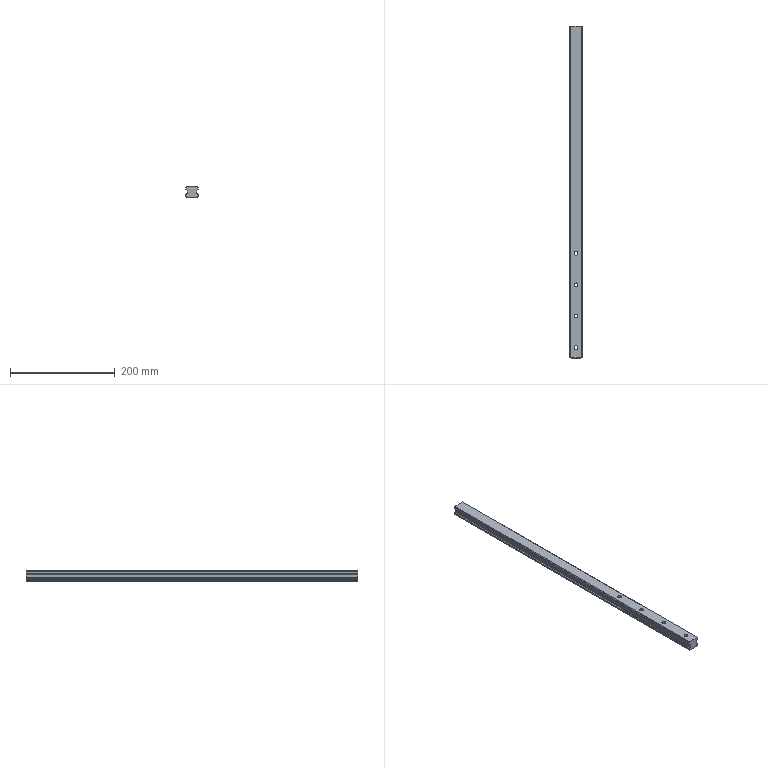Part | 1 solid | 58 faces | box 23 x 635 x 20 mm | volume 254676 mm3 | cylinder 38 | plane 20 | commonest cylinder face diameters 7 x8 11 x8 0.6 x4 0.594 x2 0.973 x2 0.985 x2